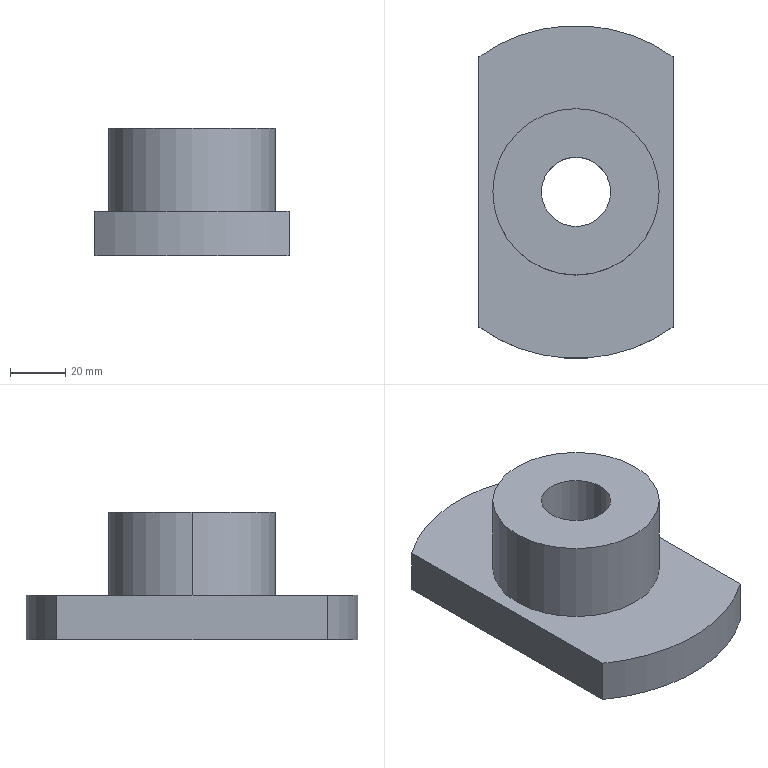Part | SolidWorks | features BaseBody 1 | 1 solid | 11 faces | box 70 x 120 x 46 mm | volume 188574 mm3 | cylinder 6 | plane 5 | commonest cylinder face diameters 25 x2 60 x2 120 x2
STEP:
#1=CARTESIAN_POINT('',(-9.453,1592.079,-1178.));
#2=VERTEX_POINT('',#1);
#3=CARTESIAN_POINT('',(-34.453,1592.079,-1178.));
#4=VERTEX_POINT('',#3);
#5=CARTESIAN_POINT('',(-21.953,1592.079,-1178.));
#6=DIRECTION('',(0.,0.,-1.));
#7=DIRECTION('',(-1.,0.,0.));
#8=AXIS2_PLACEMENT_3D('',#5,#6,#7);
#9=CIRCLE('',#8,12.5);
#10=EDGE_CURVE('',#2,#4,#9,.T.);
#11=ORIENTED_EDGE('',*,*,#10,.F.);
#12=CARTESIAN_POINT('',(-9.453,1592.079,-1224.));
#13=VERTEX_POINT('',#12);
#14=CARTESIAN_POINT('',(-9.453,1592.079,-1178.));
#15=DIRECTION('',(0.,0.,-1.));
#16=VECTOR('',#15,1000.);
#17=LINE('',#14,#16);
#18=EDGE_CURVE('',#2,#13,#17,.T.);
#19=ORIENTED_EDGE('',*,*,#18,.T.);
#20=CARTESIAN_POINT('',(-34.453,1592.079,-1224.));
#21=VERTEX_POINT('',#20);
#22=CARTESIAN_POINT('',(-21.953,1592.079,-1224.));
#23=DIRECTION('',(0.,0.,1.));
#24=DIRECTION('',(-1.,0.,0.));
#25=AXIS2_PLACEMENT_3D('',#22,#23,#24);
#26=CIRCLE('',#25,12.5);
#27=EDGE_CURVE('',#21,#13,#26,.T.);
#28=ORIENTED_EDGE('',*,*,#27,.F.);
#29=CARTESIAN_POINT('',(-34.453,1592.079,-1178.));
#30=DIRECTION('',(0.,0.,-1.));
#31=VECTOR('',#30,1000.);
#32=LINE('',#29,#31);
#33=EDGE_CURVE('',#4,#21,#32,.T.);
#34=ORIENTED_EDGE('',*,*,#33,.F.);
#35=EDGE_LOOP('',(#11,#19,#28,#34));
#36=FACE_OUTER_BOUND('',#35,.T.);
#37=CARTESIAN_POINT('',(-21.953,1592.079,-1178.));
#38=DIRECTION('',(0.,0.,-1.));
#39=DIRECTION('',(-1.,0.,0.));
#40=AXIS2_PLACEMENT_3D('',#37,#38,#39);
#41=CYLINDRICAL_SURFACE('',#40,12.5);
#42=ADVANCED_FACE('',(#36),#41,.F.);
#43=CARTESIAN_POINT('',(8.047,1592.079,-1178.));
#44=VERTEX_POINT('',#43);
#45=CARTESIAN_POINT('',(-51.953,1592.079,-1178.));
#46=VERTEX_POINT('',#45);
#47=CARTESIAN_POINT('',(-21.953,1592.079,-1178.));
#48=DIRECTION('',(0.,0.,1.));
#49=DIRECTION('',(-1.,0.,0.));
#50=AXIS2_PLACEMENT_3D('',#47,#48,#49);
#51=CIRCLE('',#50,30.);
#52=EDGE_CURVE('',#44,#46,#51,.T.);
#53=ORIENTED_EDGE('',*,*,#52,.F.);
#54=CARTESIAN_POINT('',(8.047,1592.079,-1208.));
#55=VERTEX_POINT('',#54);
#56=CARTESIAN_POINT('',(8.047,1592.079,-1178.));
#57=DIRECTION('',(0.,0.,-1.));
#58=VECTOR('',#57,1000.);
#59=LINE('',#56,#58);
#60=EDGE_CURVE('',#44,#55,#59,.T.);
#61=ORIENTED_EDGE('',*,*,#60,.T.);
#62=CARTESIAN_POINT('',(-51.953,1592.079,-1208.));
#63=VERTEX_POINT('',#62);
#64=CARTESIAN_POINT('',(-21.953,1592.079,-1208.));
#65=DIRECTION('',(0.,0.,1.));
#66=DIRECTION('',(-1.,0.,0.));
#67=AXIS2_PLACEMENT_3D('',#64,#65,#66);
#68=CIRCLE('',#67,30.);
#69=EDGE_CURVE('',#55,#63,#68,.T.);
#70=ORIENTED_EDGE('',*,*,#69,.T.);
#71=CARTESIAN_POINT('',(-51.953,1592.079,-1178.));
#72=DIRECTION('',(0.,0.,-1.));
#73=VECTOR('',#72,1000.);
#74=LINE('',#71,#73);
#75=EDGE_CURVE('',#46,#63,#74,.T.);
#76=ORIENTED_EDGE('',*,*,#75,.F.);
#77=EDGE_LOOP('',(#53,#61,#70,#76));
#78=FACE_OUTER_BOUND('',#77,.T.);
#79=CARTESIAN_POINT('',(-21.953,1592.079,-1178.));
#80=DIRECTION('',(0.,0.,-1.));
#81=DIRECTION('',(-1.,0.,0.));
#82=AXIS2_PLACEMENT_3D('',#79,#80,#81);
#83=CYLINDRICAL_SURFACE('',#82,30.);
#84=ADVANCED_FACE('',(#78),#83,.T.);
#85=ORIENTED_EDGE('',*,*,#27,.T.);
#86=CARTESIAN_POINT('',(-21.953,1592.079,-1224.));
#87=DIRECTION('',(0.,0.,1.));
#88=DIRECTION('',(-1.,0.,0.));
#89=AXIS2_PLACEMENT_3D('',#86,#87,#88);
#90=CIRCLE('',#89,12.5);
#91=EDGE_CURVE('',#13,#21,#90,.T.);
#92=ORIENTED_EDGE('',*,*,#91,.T.);
#93=EDGE_LOOP('',(#85,#92));
#94=FACE_BOUND('',#93,.T.);
#95=CARTESIAN_POINT('',(-56.953,1543.345,-1224.));
#96=VERTEX_POINT('',#95);
#97=CARTESIAN_POINT('',(-56.953,1640.813,-1224.));
#98=VERTEX_POINT('',#97);
#99=CARTESIAN_POINT('',(-56.953,1592.079,-1224.));
#100=DIRECTION('',(0.,1.,0.));
#101=VECTOR('',#100,1000.);
#102=LINE('',#99,#101);
#103=EDGE_CURVE('',#96,#98,#102,.T.);
#104=ORIENTED_EDGE('',*,*,#103,.T.);
#105=CARTESIAN_POINT('',(13.047,1640.813,-1224.));
#106=VERTEX_POINT('',#105);
#107=CARTESIAN_POINT('',(-21.953,1592.079,-1224.));
#108=DIRECTION('',(0.,0.,-1.));
#109=DIRECTION('',(1.,0.,0.));
#110=AXIS2_PLACEMENT_3D('',#107,#108,#109);
#111=CIRCLE('',#110,60.);
#112=EDGE_CURVE('',#98,#106,#111,.T.);
#113=ORIENTED_EDGE('',*,*,#112,.T.);
#114=CARTESIAN_POINT('',(13.047,1543.345,-1224.));
#115=VERTEX_POINT('',#114);
#116=CARTESIAN_POINT('',(13.047,1592.079,-1224.));
#117=DIRECTION('',(0.,-1.,0.));
#118=VECTOR('',#117,1000.);
#119=LINE('',#116,#118);
#120=EDGE_CURVE('',#106,#115,#119,.T.);
#121=ORIENTED_EDGE('',*,*,#120,.T.);
#122=CARTESIAN_POINT('',(-21.953,1592.079,-1224.));
#123=DIRECTION('',(0.,0.,-1.));
#124=DIRECTION('',(1.,0.,0.));
#125=AXIS2_PLACEMENT_3D('',#122,#123,#124);
#126=CIRCLE('',#125,60.);
#127=EDGE_CURVE('',#115,#96,#126,.T.);
#128=ORIENTED_EDGE('',*,*,#127,.T.);
#129=EDGE_LOOP('',(#104,#113,#121,#128));
#130=FACE_OUTER_BOUND('',#129,.T.);
#131=CARTESIAN_POINT('',(-21.953,1592.079,-1224.));
#132=DIRECTION('',(0.,0.,-1.));
#133=DIRECTION('',(-1.,0.,0.));
#134=AXIS2_PLACEMENT_3D('',#131,#132,#133);
#135=PLANE('',#134);
#136=ADVANCED_FACE('',(#94,#130),#135,.T.);
#137=ORIENTED_EDGE('',*,*,#18,.F.);
#138=CARTESIAN_POINT('',(-21.953,1592.079,-1178.));
#139=DIRECTION('',(0.,0.,-1.));
#140=DIRECTION('',(-1.,0.,0.));
#141=AXIS2_PLACEMENT_3D('',#138,#139,#140);
#142=CIRCLE('',#141,12.5);
#143=EDGE_CURVE('',#4,#2,#142,.T.);
#144=ORIENTED_EDGE('',*,*,#143,.F.);
#145=ORIENTED_EDGE('',*,*,#33,.T.);
#146=ORIENTED_EDGE('',*,*,#91,.F.);
#147=EDGE_LOOP('',(#137,#144,#145,#146));
#148=FACE_OUTER_BOUND('',#147,.T.);
#149=CARTESIAN_POINT('',(-21.953,1592.079,-1178.));
#150=DIRECTION('',(0.,0.,-1.));
#151=DIRECTION('',(-1.,0.,0.));
#152=AXIS2_PLACEMENT_3D('',#149,#150,#151);
#153=CYLINDRICAL_SURFACE('',#152,12.5);
#154=ADVANCED_FACE('',(#148),#153,.F.);
#155=CARTESIAN_POINT('',(-56.953,1640.813,-1208.));
#156=VERTEX_POINT('',#155);
#157=CARTESIAN_POINT('',(-56.953,1640.813,-1224.));
#158=DIRECTION('',(0.,0.,1.));
#159=VECTOR('',#158,1000.);
#160=LINE('',#157,#159);
#161=EDGE_CURVE('',#98,#156,#160,.T.);
#162=ORIENTED_EDGE('',*,*,#161,.T.);
#163=CARTESIAN_POINT('',(13.047,1640.813,-1208.));
#164=VERTEX_POINT('',#163);
#165=CARTESIAN_POINT('',(-21.953,1592.079,-1208.));
#166=DIRECTION('',(0.,0.,-1.));
#167=DIRECTION('',(1.,0.,0.));
#168=AXIS2_PLACEMENT_3D('',#165,#166,#167);
#169=CIRCLE('',#168,60.);
#170=EDGE_CURVE('',#156,#164,#169,.T.);
#171=ORIENTED_EDGE('',*,*,#170,.T.);
#172=CARTESIAN_POINT('',(13.047,1640.813,-1224.));
#173=DIRECTION('',(0.,0.,-1.));
#174=VECTOR('',#173,1000.);
#175=LINE('',#172,#174);
#176=EDGE_CURVE('',#164,#106,#175,.T.);
#177=ORIENTED_EDGE('',*,*,#176,.T.);
#178=ORIENTED_EDGE('',*,*,#112,.F.);
#179=EDGE_LOOP('',(#162,#171,#177,#178));
#180=FACE_OUTER_BOUND('',#179,.T.);
#181=CARTESIAN_POINT('',(-21.953,1592.079,-1224.));
#182=DIRECTION('',(0.,0.,1.));
#183=DIRECTION('',(1.,0.,0.));
#184=AXIS2_PLACEMENT_3D('',#181,#182,#183);
#185=CYLINDRICAL_SURFACE('',#184,60.);
#186=ADVANCED_FACE('',(#180),#185,.T.);
#187=ORIENTED_EDGE('',*,*,#103,.F.);
#188=CARTESIAN_POINT('',(-56.953,1543.345,-1208.));
#189=VERTEX_POINT('',#188);
#190=CARTESIAN_POINT('',(-56.953,1543.345,-1224.));
#191=DIRECTION('',(0.,0.,-1.));
#192=VECTOR('',#191,1000.);
#193=LINE('',#190,#192);
#194=EDGE_CURVE('',#189,#96,#193,.T.);
#195=ORIENTED_EDGE('',*,*,#194,.F.);
#196=CARTESIAN_POINT('',(-56.953,1640.813,-1208.));
#197=DIRECTION('',(0.,-1.,0.));
#198=VECTOR('',#197,1000.);
#199=LINE('',#196,#198);
#200=EDGE_CURVE('',#156,#189,#199,.T.);
#201=ORIENTED_EDGE('',*,*,#200,.F.);
#202=ORIENTED_EDGE('',*,*,#161,.F.);
#203=EDGE_LOOP('',(#187,#195,#201,#202));
#204=FACE_OUTER_BOUND('',#203,.T.);
#205=CARTESIAN_POINT('',(-56.953,1640.813,-1224.));
#206=DIRECTION('',(1.,0.,0.));
#207=DIRECTION('',(0.,0.,-1.));
#208=AXIS2_PLACEMENT_3D('',#205,#206,#207);
#209=PLANE('',#208);
#210=ADVANCED_FACE('',(#204),#209,.F.);
#211=CARTESIAN_POINT('',(13.047,1543.345,-1208.));
#212=VERTEX_POINT('',#211);
#213=CARTESIAN_POINT('',(13.047,1543.345,-1224.));
#214=DIRECTION('',(0.,0.,1.));
#215=VECTOR('',#214,1000.);
#216=LINE('',#213,#215);
#217=EDGE_CURVE('',#115,#212,#216,.T.);
#218=ORIENTED_EDGE('',*,*,#217,.T.);
#219=CARTESIAN_POINT('',(-21.953,1592.079,-1208.));
#220=DIRECTION('',(0.,0.,-1.));
#221=DIRECTION('',(1.,0.,0.));
#222=AXIS2_PLACEMENT_3D('',#219,#220,#221);
#223=CIRCLE('',#222,60.);
#224=EDGE_CURVE('',#212,#189,#223,.T.);
#225=ORIENTED_EDGE('',*,*,#224,.T.);
#226=ORIENTED_EDGE('',*,*,#194,.T.);
#227=ORIENTED_EDGE('',*,*,#127,.F.);
#228=EDGE_LOOP('',(#218,#225,#226,#227));
#229=FACE_OUTER_BOUND('',#228,.T.);
#230=CARTESIAN_POINT('',(-21.953,1592.079,-1224.));
#231=DIRECTION('',(0.,0.,1.));
#232=DIRECTION('',(1.,0.,0.));
#233=AXIS2_PLACEMENT_3D('',#230,#231,#232);
#234=CYLINDRICAL_SURFACE('',#233,60.);
#235=ADVANCED_FACE('',(#229),#234,.T.);
#236=ORIENTED_EDGE('',*,*,#120,.F.);
#237=ORIENTED_EDGE('',*,*,#176,.F.);
#238=CARTESIAN_POINT('',(13.047,1640.813,-1208.));
#239=DIRECTION('',(0.,1.,0.));
#240=VECTOR('',#239,1000.);
#241=LINE('',#238,#240);
#242=EDGE_CURVE('',#212,#164,#241,.T.);
#243=ORIENTED_EDGE('',*,*,#242,.F.);
#244=ORIENTED_EDGE('',*,*,#217,.F.);
#245=EDGE_LOOP('',(#236,#237,#243,#244));
#246=FACE_OUTER_BOUND('',#245,.T.);
#247=CARTESIAN_POINT('',(13.047,1640.813,-1224.));
#248=DIRECTION('',(-1.,0.,0.));
#249=DIRECTION('',(0.,0.,1.));
#250=AXIS2_PLACEMENT_3D('',#247,#248,#249);
#251=PLANE('',#250);
#252=ADVANCED_FACE('',(#246),#251,.F.);
#253=ORIENTED_EDGE('',*,*,#143,.T.);
#254=ORIENTED_EDGE('',*,*,#10,.T.);
#255=EDGE_LOOP('',(#253,#254));
#256=FACE_BOUND('',#255,.T.);
#257=CARTESIAN_POINT('',(-21.953,1592.079,-1178.));
#258=DIRECTION('',(0.,0.,1.));
#259=DIRECTION('',(-1.,0.,0.));
#260=AXIS2_PLACEMENT_3D('',#257,#258,#259);
#261=CIRCLE('',#260,30.);
#262=EDGE_CURVE('',#46,#44,#261,.T.);
#263=ORIENTED_EDGE('',*,*,#262,.T.);
#264=ORIENTED_EDGE('',*,*,#52,.T.);
#265=EDGE_LOOP('',(#263,#264));
#266=FACE_OUTER_BOUND('',#265,.T.);
#267=CARTESIAN_POINT('',(-21.953,1592.079,-1178.));
#268=DIRECTION('',(0.,0.,1.));
#269=DIRECTION('',(1.,0.,0.));
#270=AXIS2_PLACEMENT_3D('',#267,#268,#269);
#271=PLANE('',#270);
#272=ADVANCED_FACE('',(#256,#266),#271,.T.);
#273=CARTESIAN_POINT('',(-21.953,1592.079,-1208.));
#274=DIRECTION('',(0.,0.,1.));
#275=DIRECTION('',(-1.,0.,0.));
#276=AXIS2_PLACEMENT_3D('',#273,#274,#275);
#277=CIRCLE('',#276,30.);
#278=EDGE_CURVE('',#63,#55,#277,.T.);
#279=ORIENTED_EDGE('',*,*,#278,.F.);
#280=ORIENTED_EDGE('',*,*,#69,.F.);
#281=EDGE_LOOP('',(#279,#280));
#282=FACE_BOUND('',#281,.T.);
#283=ORIENTED_EDGE('',*,*,#200,.T.);
#284=ORIENTED_EDGE('',*,*,#224,.F.);
#285=ORIENTED_EDGE('',*,*,#242,.T.);
#286=ORIENTED_EDGE('',*,*,#170,.F.);
#287=EDGE_LOOP('',(#283,#284,#285,#286));
#288=FACE_OUTER_BOUND('',#287,.T.);
#289=CARTESIAN_POINT('',(-21.953,1592.079,-1208.));
#290=DIRECTION('',(0.,0.,-1.));
#291=DIRECTION('',(-1.,0.,0.));
#292=AXIS2_PLACEMENT_3D('',#289,#290,#291);
#293=PLANE('',#292);
#294=ADVANCED_FACE('',(#282,#288),#293,.F.);
#295=ORIENTED_EDGE('',*,*,#60,.F.);
#296=ORIENTED_EDGE('',*,*,#262,.F.);
#297=ORIENTED_EDGE('',*,*,#75,.T.);
#298=ORIENTED_EDGE('',*,*,#278,.T.);
#299=EDGE_LOOP('',(#295,#296,#297,#298));
#300=FACE_OUTER_BOUND('',#299,.T.);
#301=CARTESIAN_POINT('',(-21.953,1592.079,-1178.));
#302=DIRECTION('',(0.,0.,-1.));
#303=DIRECTION('',(-1.,0.,0.));
#304=AXIS2_PLACEMENT_3D('',#301,#302,#303);
#305=CYLINDRICAL_SURFACE('',#304,30.);
#306=ADVANCED_FACE('',(#300),#305,.T.);
#307=CLOSED_SHELL('',(#42,#84,#136,#154,#186,#210,#235,#252,#272,#294,#306));
#308=MANIFOLD_SOLID_BREP('',#307);
#309=CARTESIAN_POINT('',(0.,0.,0.));
#310=DIRECTION('',(0.,0.,1.));
#311=DIRECTION('',(1.,0.,0.));
#312=AXIS2_PLACEMENT_3D('',#309,#310,#311);
#313=(LENGTH_UNIT()NAMED_UNIT(*)SI_UNIT(.MILLI.,.METRE.));
#314=UNCERTAINTY_MEASURE_WITH_UNIT(LENGTH_MEASURE(0.00001),#313,'','');
#315=(NAMED_UNIT(*)PLANE_ANGLE_UNIT()SI_UNIT($,.RADIAN.));
#316=(NAMED_UNIT(*)SI_UNIT($,.STERADIAN.)SOLID_ANGLE_UNIT());
#317=(GEOMETRIC_REPRESENTATION_CONTEXT(3)GLOBAL_UNCERTAINTY_ASSIGNED_CONTEXT((#314))GLOBAL_UNIT_ASSIGNED_CONTEXT((#313,#315,#316))REPRESENTATION_CONTEXT('',''));
#318=ADVANCED_BREP_SHAPE_REPRESENTATION('',(#308,#312),#317);